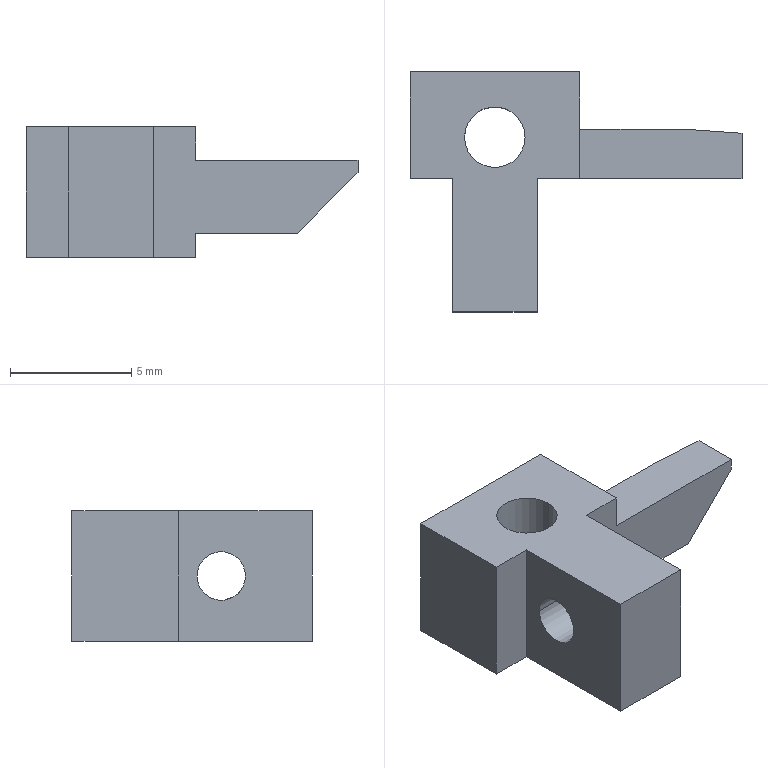Part | NX | 1 solid | 23 faces | box 13.7 x 9.913 x 5.4 mm | volume 252.029 mm3 | plane 17 | cylinder 6 | commonest cylinder face diameters 2 x2 2.5 x2 3.1 x2
STEP:
#1=CARTESIAN_POINT('',(-48.11,-45.316,4.403));
#2=VERTEX_POINT('',#1);
#3=CARTESIAN_POINT('',(-55.11,-45.316,4.403));
#4=VERTEX_POINT('',#3);
#5=CARTESIAN_POINT('',(-48.11,-45.316,4.403));
#6=DIRECTION('',(-1.,0.,0.));
#7=VECTOR('',#6,1000.);
#8=LINE('',#5,#7);
#9=EDGE_CURVE('',#2,#4,#8,.T.);
#10=ORIENTED_EDGE('',*,*,#9,.F.);
#11=CARTESIAN_POINT('',(-48.11,-45.316,-0.9969));
#12=VERTEX_POINT('',#11);
#13=CARTESIAN_POINT('',(-48.11,-45.316,4.403));
#14=DIRECTION('',(0.,0.,-1.));
#15=VECTOR('',#14,1000.);
#16=LINE('',#13,#15);
#17=EDGE_CURVE('',#2,#12,#16,.T.);
#18=ORIENTED_EDGE('',*,*,#17,.T.);
#19=CARTESIAN_POINT('',(-55.11,-45.316,-0.9969));
#20=VERTEX_POINT('',#19);
#21=CARTESIAN_POINT('',(-49.101,-45.316,-0.9969));
#22=DIRECTION('',(-1.,0.,0.));
#23=VECTOR('',#22,1000.);
#24=LINE('',#21,#23);
#25=EDGE_CURVE('',#12,#20,#24,.T.);
#26=ORIENTED_EDGE('',*,*,#25,.T.);
#27=CARTESIAN_POINT('',(-55.11,-45.316,4.403));
#28=DIRECTION('',(0.,0.,-1.));
#29=VECTOR('',#28,1000.);
#30=LINE('',#27,#29);
#31=EDGE_CURVE('',#4,#20,#30,.T.);
#32=ORIENTED_EDGE('',*,*,#31,.F.);
#33=EDGE_LOOP('',(#10,#18,#26,#32));
#34=FACE_BOUND('',#33,.T.);
#35=CARTESIAN_POINT('',(-48.11,-45.316,4.403));
#36=DIRECTION('',(0.,1.,0.));
#37=DIRECTION('',(0.,0.,-1.));
#38=AXIS2_PLACEMENT_3D('',#35,#36,#37);
#39=PLANE('',#38);
#40=ADVANCED_FACE('',(#34),#39,.T.);
#41=CARTESIAN_POINT('',(-48.11,-49.729,-0.9969));
#42=VERTEX_POINT('',#41);
#43=CARTESIAN_POINT('',(-48.11,-51.163,-0.9969));
#44=DIRECTION('',(0.,1.,0.));
#45=VECTOR('',#44,1000.);
#46=LINE('',#43,#45);
#47=EDGE_CURVE('',#42,#12,#46,.T.);
#48=ORIENTED_EDGE('',*,*,#47,.F.);
#49=CARTESIAN_POINT('',(-49.86,-49.729,-0.9969));
#50=VERTEX_POINT('',#49);
#51=CARTESIAN_POINT('',(-49.101,-49.729,-0.9969));
#52=DIRECTION('',(-1.,0.,0.));
#53=VECTOR('',#52,1000.);
#54=LINE('',#51,#53);
#55=EDGE_CURVE('',#42,#50,#54,.T.);
#56=ORIENTED_EDGE('',*,*,#55,.T.);
#57=CARTESIAN_POINT('',(-49.86,-55.229,-0.9969));
#58=VERTEX_POINT('',#57);
#59=CARTESIAN_POINT('',(-49.86,-51.163,-0.9969));
#60=DIRECTION('',(0.,-1.,0.));
#61=VECTOR('',#60,1000.);
#62=LINE('',#59,#61);
#63=EDGE_CURVE('',#50,#58,#62,.T.);
#64=ORIENTED_EDGE('',*,*,#63,.T.);
#65=CARTESIAN_POINT('',(-53.36,-55.229,-0.9969));
#66=VERTEX_POINT('',#65);
#67=CARTESIAN_POINT('',(-49.86,-55.229,-0.9969));
#68=DIRECTION('',(-1.,0.,0.));
#69=VECTOR('',#68,1000.);
#70=LINE('',#67,#69);
#71=EDGE_CURVE('',#58,#66,#70,.T.);
#72=ORIENTED_EDGE('',*,*,#71,.T.);
#73=CARTESIAN_POINT('',(-53.36,-49.729,-0.9969));
#74=VERTEX_POINT('',#73);
#75=CARTESIAN_POINT('',(-53.36,-51.163,-0.9969));
#76=DIRECTION('',(0.,-1.,0.));
#77=VECTOR('',#76,1000.);
#78=LINE('',#75,#77);
#79=EDGE_CURVE('',#74,#66,#78,.T.);
#80=ORIENTED_EDGE('',*,*,#79,.F.);
#81=CARTESIAN_POINT('',(-55.11,-49.729,-0.9969));
#82=VERTEX_POINT('',#81);
#83=CARTESIAN_POINT('',(-49.101,-49.729,-0.9969));
#84=DIRECTION('',(-1.,0.,0.));
#85=VECTOR('',#84,1000.);
#86=LINE('',#83,#85);
#87=EDGE_CURVE('',#74,#82,#86,.T.);
#88=ORIENTED_EDGE('',*,*,#87,.T.);
#89=CARTESIAN_POINT('',(-55.11,-51.163,-0.9969));
#90=DIRECTION('',(0.,1.,0.));
#91=VECTOR('',#90,1000.);
#92=LINE('',#89,#91);
#93=EDGE_CURVE('',#82,#20,#92,.T.);
#94=ORIENTED_EDGE('',*,*,#93,.T.);
#95=ORIENTED_EDGE('',*,*,#25,.F.);
#96=EDGE_LOOP('',(#48,#56,#64,#72,#80,#88,#94,#95));
#97=FACE_BOUND('',#96,.T.);
#98=CARTESIAN_POINT('',(-50.06,-53.51,-0.9969));
#99=VERTEX_POINT('',#98);
#100=CARTESIAN_POINT('',(-53.16,-53.51,-0.9969));
#101=VERTEX_POINT('',#100);
#102=CARTESIAN_POINT('',(-51.61,-53.51,-0.9969));
#103=DIRECTION('',(0.,0.,-1.));
#104=DIRECTION('',(-1.,0.,0.));
#105=AXIS2_PLACEMENT_3D('',#102,#103,#104);
#106=CIRCLE('',#105,1.55);
#107=EDGE_CURVE('',#99,#101,#106,.T.);
#108=ORIENTED_EDGE('',*,*,#107,.F.);
#109=CARTESIAN_POINT('',(-51.61,-53.51,-0.9969));
#110=DIRECTION('',(0.,0.,-1.));
#111=DIRECTION('',(-1.,0.,0.));
#112=AXIS2_PLACEMENT_3D('',#109,#110,#111);
#113=CIRCLE('',#112,1.55);
#114=EDGE_CURVE('',#101,#99,#113,.T.);
#115=ORIENTED_EDGE('',*,*,#114,.F.);
#116=EDGE_LOOP('',(#108,#115));
#117=FACE_BOUND('',#116,.T.);
#118=CARTESIAN_POINT('',(-52.86,-48.012,-0.9969));
#119=VERTEX_POINT('',#118);
#120=CARTESIAN_POINT('',(-50.36,-48.012,-0.9969));
#121=VERTEX_POINT('',#120);
#122=CARTESIAN_POINT('',(-51.61,-48.012,-0.9969));
#123=DIRECTION('',(0.,0.,-1.));
#124=DIRECTION('',(-1.,0.,0.));
#125=AXIS2_PLACEMENT_3D('',#122,#123,#124);
#126=CIRCLE('',#125,1.25);
#127=EDGE_CURVE('',#119,#121,#126,.T.);
#128=ORIENTED_EDGE('',*,*,#127,.F.);
#129=CARTESIAN_POINT('',(-51.61,-48.012,-0.9969));
#130=DIRECTION('',(0.,0.,-1.));
#131=DIRECTION('',(-1.,0.,0.));
#132=AXIS2_PLACEMENT_3D('',#129,#130,#131);
#133=CIRCLE('',#132,1.25);
#134=EDGE_CURVE('',#121,#119,#133,.T.);
#135=ORIENTED_EDGE('',*,*,#134,.F.);
#136=EDGE_LOOP('',(#128,#135));
#137=FACE_BOUND('',#136,.T.);
#138=CARTESIAN_POINT('',(-49.101,-51.163,-0.9969));
#139=DIRECTION('',(0.,0.,-1.));
#140=DIRECTION('',(0.,-1.,0.));
#141=AXIS2_PLACEMENT_3D('',#138,#139,#140);
#142=PLANE('',#141);
#143=ADVANCED_FACE('',(#97,#117,#137),#142,.T.);
#144=ORIENTED_EDGE('',*,*,#47,.T.);
#145=ORIENTED_EDGE('',*,*,#17,.F.);
#146=CARTESIAN_POINT('',(-48.11,-49.729,4.403));
#147=VERTEX_POINT('',#146);
#148=CARTESIAN_POINT('',(-48.11,-51.163,4.403));
#149=DIRECTION('',(0.,1.,0.));
#150=VECTOR('',#149,1000.);
#151=LINE('',#148,#150);
#152=EDGE_CURVE('',#147,#2,#151,.T.);
#153=ORIENTED_EDGE('',*,*,#152,.F.);
#154=CARTESIAN_POINT('',(-48.11,-49.729,3.003));
#155=VERTEX_POINT('',#154);
#156=CARTESIAN_POINT('',(-48.11,-49.729,4.403));
#157=DIRECTION('',(0.,0.,-1.));
#158=VECTOR('',#157,1000.);
#159=LINE('',#156,#158);
#160=EDGE_CURVE('',#147,#155,#159,.T.);
#161=ORIENTED_EDGE('',*,*,#160,.T.);
#162=CARTESIAN_POINT('',(-48.11,-47.687,3.003));
#163=VERTEX_POINT('',#162);
#164=CARTESIAN_POINT('',(-48.11,-51.163,3.003));
#165=DIRECTION('',(0.,-1.,0.));
#166=VECTOR('',#165,1000.);
#167=LINE('',#164,#166);
#168=EDGE_CURVE('',#163,#155,#167,.T.);
#169=ORIENTED_EDGE('',*,*,#168,.F.);
#170=CARTESIAN_POINT('',(-48.11,-47.687,0.003122));
#171=VERTEX_POINT('',#170);
#172=CARTESIAN_POINT('',(-48.11,-47.687,4.403));
#173=DIRECTION('',(0.,0.,1.));
#174=VECTOR('',#173,1000.);
#175=LINE('',#172,#174);
#176=EDGE_CURVE('',#171,#163,#175,.T.);
#177=ORIENTED_EDGE('',*,*,#176,.F.);
#178=CARTESIAN_POINT('',(-48.11,-49.729,0.003122));
#179=VERTEX_POINT('',#178);
#180=CARTESIAN_POINT('',(-48.11,-51.163,0.003122));
#181=DIRECTION('',(0.,1.,0.));
#182=VECTOR('',#181,1000.);
#183=LINE('',#180,#182);
#184=EDGE_CURVE('',#179,#171,#183,.T.);
#185=ORIENTED_EDGE('',*,*,#184,.F.);
#186=CARTESIAN_POINT('',(-48.11,-49.729,4.403));
#187=DIRECTION('',(0.,0.,-1.));
#188=VECTOR('',#187,1000.);
#189=LINE('',#186,#188);
#190=EDGE_CURVE('',#179,#42,#189,.T.);
#191=ORIENTED_EDGE('',*,*,#190,.T.);
#192=EDGE_LOOP('',(#144,#145,#153,#161,#169,#177,#185,#191));
#193=FACE_BOUND('',#192,.T.);
#194=CARTESIAN_POINT('',(-48.11,-47.529,-0.5969));
#195=DIRECTION('',(1.,0.,0.));
#196=DIRECTION('',(0.,1.,0.));
#197=AXIS2_PLACEMENT_3D('',#194,#195,#196);
#198=PLANE('',#197);
#199=ADVANCED_FACE('',(#193),#198,.T.);
#200=CARTESIAN_POINT('',(-55.11,-49.729,4.403));
#201=VERTEX_POINT('',#200);
#202=CARTESIAN_POINT('',(-55.11,-49.729,4.403));
#203=DIRECTION('',(0.,0.,1.));
#204=VECTOR('',#203,1000.);
#205=LINE('',#202,#204);
#206=EDGE_CURVE('',#82,#201,#205,.T.);
#207=ORIENTED_EDGE('',*,*,#206,.T.);
#208=CARTESIAN_POINT('',(-55.11,-51.163,4.403));
#209=DIRECTION('',(0.,-1.,0.));
#210=VECTOR('',#209,1000.);
#211=LINE('',#208,#210);
#212=EDGE_CURVE('',#4,#201,#211,.T.);
#213=ORIENTED_EDGE('',*,*,#212,.F.);
#214=ORIENTED_EDGE('',*,*,#31,.T.);
#215=ORIENTED_EDGE('',*,*,#93,.F.);
#216=EDGE_LOOP('',(#207,#213,#214,#215));
#217=FACE_BOUND('',#216,.T.);
#218=CARTESIAN_POINT('',(-55.11,-45.316,-0.5969));
#219=DIRECTION('',(-1.,0.,0.));
#220=DIRECTION('',(0.,0.,1.));
#221=AXIS2_PLACEMENT_3D('',#218,#219,#220);
#222=PLANE('',#221);
#223=ADVANCED_FACE('',(#217),#222,.T.);
#224=CARTESIAN_POINT('',(-43.739,-47.687,3.003));
#225=VERTEX_POINT('',#224);
#226=CARTESIAN_POINT('',(-49.101,-47.687,3.003));
#227=DIRECTION('',(1.,0.,0.));
#228=VECTOR('',#227,1000.);
#229=LINE('',#226,#228);
#230=EDGE_CURVE('',#163,#225,#229,.T.);
#231=ORIENTED_EDGE('',*,*,#230,.F.);
#232=ORIENTED_EDGE('',*,*,#168,.T.);
#233=CARTESIAN_POINT('',(-41.41,-49.729,3.003));
#234=VERTEX_POINT('',#233);
#235=CARTESIAN_POINT('',(-49.101,-49.729,3.003));
#236=DIRECTION('',(1.,0.,0.));
#237=VECTOR('',#236,1000.);
#238=LINE('',#235,#237);
#239=EDGE_CURVE('',#155,#234,#238,.T.);
#240=ORIENTED_EDGE('',*,*,#239,.T.);
#241=CARTESIAN_POINT('',(-41.41,-47.851,3.003));
#242=VERTEX_POINT('',#241);
#243=CARTESIAN_POINT('',(-41.41,-51.163,3.003));
#244=DIRECTION('',(0.,1.,0.));
#245=VECTOR('',#244,1000.);
#246=LINE('',#243,#245);
#247=EDGE_CURVE('',#234,#242,#246,.T.);
#248=ORIENTED_EDGE('',*,*,#247,.T.);
#249=CARTESIAN_POINT('',(-49.101,-47.307,3.003));
#250=DIRECTION('',(0.9975,-0.07053,0.));
#251=VECTOR('',#250,1000.);
#252=LINE('',#249,#251);
#253=EDGE_CURVE('',#225,#242,#252,.T.);
#254=ORIENTED_EDGE('',*,*,#253,.F.);
#255=EDGE_LOOP('',(#231,#232,#240,#248,#254));
#256=FACE_BOUND('',#255,.T.);
#257=CARTESIAN_POINT('',(-48.11,-53.629,3.003));
#258=DIRECTION('',(0.,0.,1.));
#259=DIRECTION('',(1.,0.,0.));
#260=AXIS2_PLACEMENT_3D('',#257,#258,#259);
#261=PLANE('',#260);
#262=ADVANCED_FACE('',(#256),#261,.T.);
#263=ORIENTED_EDGE('',*,*,#127,.T.);
#264=CARTESIAN_POINT('',(-50.36,-48.012,4.403));
#265=VERTEX_POINT('',#264);
#266=CARTESIAN_POINT('',(-50.36,-48.012,-2.597));
#267=DIRECTION('',(0.,0.,-1.));
#268=VECTOR('',#267,1000.);
#269=LINE('',#266,#268);
#270=EDGE_CURVE('',#265,#121,#269,.T.);
#271=ORIENTED_EDGE('',*,*,#270,.F.);
#272=CARTESIAN_POINT('',(-52.86,-48.012,4.403));
#273=VERTEX_POINT('',#272);
#274=CARTESIAN_POINT('',(-51.61,-48.012,4.403));
#275=DIRECTION('',(0.,0.,-1.));
#276=DIRECTION('',(-1.,0.,0.));
#277=AXIS2_PLACEMENT_3D('',#274,#275,#276);
#278=CIRCLE('',#277,1.25);
#279=EDGE_CURVE('',#273,#265,#278,.T.);
#280=ORIENTED_EDGE('',*,*,#279,.F.);
#281=CARTESIAN_POINT('',(-52.86,-48.012,-2.597));
#282=DIRECTION('',(0.,0.,-1.));
#283=VECTOR('',#282,1000.);
#284=LINE('',#281,#283);
#285=EDGE_CURVE('',#273,#119,#284,.T.);
#286=ORIENTED_EDGE('',*,*,#285,.T.);
#287=EDGE_LOOP('',(#263,#271,#280,#286));
#288=FACE_BOUND('',#287,.T.);
#289=CARTESIAN_POINT('',(-51.61,-48.012,-2.597));
#290=DIRECTION('',(0.,0.,-1.));
#291=DIRECTION('',(-1.,0.,0.));
#292=AXIS2_PLACEMENT_3D('',#289,#290,#291);
#293=CYLINDRICAL_SURFACE('',#292,1.25);
#294=ADVANCED_FACE('',(#288),#293,.F.);
#295=ORIENTED_EDGE('',*,*,#230,.T.);
#296=CARTESIAN_POINT('',(-46.739,-47.687,0.003122));
#297=VERTEX_POINT('',#296);
#298=CARTESIAN_POINT('',(-44.574,-47.687,2.167));
#299=DIRECTION('',(0.7071,0.,0.7071));
#300=VECTOR('',#299,1000.);
#301=LINE('',#298,#300);
#302=EDGE_CURVE('',#297,#225,#301,.T.);
#303=ORIENTED_EDGE('',*,*,#302,.F.);
#304=CARTESIAN_POINT('',(-49.101,-47.687,0.003122));
#305=DIRECTION('',(-1.,0.,0.));
#306=VECTOR('',#305,1000.);
#307=LINE('',#304,#306);
#308=EDGE_CURVE('',#297,#171,#307,.T.);
#309=ORIENTED_EDGE('',*,*,#308,.T.);
#310=ORIENTED_EDGE('',*,*,#176,.T.);
#311=EDGE_LOOP('',(#295,#303,#309,#310));
#312=FACE_BOUND('',#311,.T.);
#313=CARTESIAN_POINT('',(-48.11,-47.687,2.503));
#314=DIRECTION('',(0.,1.,0.));
#315=DIRECTION('',(1.,0.,0.));
#316=AXIS2_PLACEMENT_3D('',#313,#314,#315);
#317=PLANE('',#316);
#318=ADVANCED_FACE('',(#312),#317,.T.);
#319=ORIENTED_EDGE('',*,*,#87,.F.);
#320=CARTESIAN_POINT('',(-53.36,-49.729,4.403));
#321=VERTEX_POINT('',#320);
#322=CARTESIAN_POINT('',(-53.36,-49.729,4.403));
#323=DIRECTION('',(0.,0.,1.));
#324=VECTOR('',#323,1000.);
#325=LINE('',#322,#324);
#326=EDGE_CURVE('',#74,#321,#325,.T.);
#327=ORIENTED_EDGE('',*,*,#326,.T.);
#328=CARTESIAN_POINT('',(-49.101,-49.729,4.403));
#329=DIRECTION('',(-1.,0.,0.));
#330=VECTOR('',#329,1000.);
#331=LINE('',#328,#330);
#332=EDGE_CURVE('',#321,#201,#331,.T.);
#333=ORIENTED_EDGE('',*,*,#332,.T.);
#334=ORIENTED_EDGE('',*,*,#206,.F.);
#335=EDGE_LOOP('',(#319,#327,#333,#334));
#336=FACE_BOUND('',#335,.T.);
#337=CARTESIAN_POINT('',(-48.11,-49.729,-0.5969));
#338=DIRECTION('',(0.,-1.,0.));
#339=DIRECTION('',(0.,0.,-1.));
#340=AXIS2_PLACEMENT_3D('',#337,#338,#339);
#341=PLANE('',#340);
#342=ADVANCED_FACE('',(#336),#341,.T.);
#343=CARTESIAN_POINT('',(-41.41,-49.729,2.503));
#344=VERTEX_POINT('',#343);
#345=CARTESIAN_POINT('',(-41.41,-47.887,2.503));
#346=VERTEX_POINT('',#345);
#347=CARTESIAN_POINT('',(-41.41,-51.163,2.503));
#348=DIRECTION('',(0.,1.,0.));
#349=VECTOR('',#348,1000.);
#350=LINE('',#347,#349);
#351=EDGE_CURVE('',#344,#346,#350,.T.);
#352=ORIENTED_EDGE('',*,*,#351,.T.);
#353=CARTESIAN_POINT('',(-41.41,-47.752,4.403));
#354=DIRECTION('',(0.,-0.07053,-0.9975));
#355=VECTOR('',#354,1000.);
#356=LINE('',#353,#355);
#357=EDGE_CURVE('',#242,#346,#356,.T.);
#358=ORIENTED_EDGE('',*,*,#357,.F.);
#359=ORIENTED_EDGE('',*,*,#247,.F.);
#360=CARTESIAN_POINT('',(-41.41,-49.729,4.403));
#361=DIRECTION('',(0.,0.,-1.));
#362=VECTOR('',#361,1000.);
#363=LINE('',#360,#362);
#364=EDGE_CURVE('',#234,#344,#363,.T.);
#365=ORIENTED_EDGE('',*,*,#364,.T.);
#366=EDGE_LOOP('',(#352,#358,#359,#365));
#367=FACE_BOUND('',#366,.T.);
#368=CARTESIAN_POINT('',(-41.41,-49.37,2.047));
#369=DIRECTION('',(1.,0.,0.));
#370=DIRECTION('',(0.,1.,0.));
#371=AXIS2_PLACEMENT_3D('',#368,#369,#370);
#372=PLANE('',#371);
#373=ADVANCED_FACE('',(#367),#372,.T.);
#374=CARTESIAN_POINT('',(-43.91,-47.887,0.003122));
#375=VERTEX_POINT('',#374);
#376=CARTESIAN_POINT('',(-43.16,-47.887,0.7531));
#377=DIRECTION('',(0.7071,0.,0.7071));
#378=VECTOR('',#377,1000.);
#379=LINE('',#376,#378);
#380=EDGE_CURVE('',#375,#346,#379,.T.);
#381=ORIENTED_EDGE('',*,*,#380,.T.);
#382=ORIENTED_EDGE('',*,*,#351,.F.);
#383=CARTESIAN_POINT('',(-43.91,-49.729,0.003122));
#384=VERTEX_POINT('',#383);
#385=CARTESIAN_POINT('',(-39.51,-49.729,4.403));
#386=DIRECTION('',(-0.7071,0.,-0.7071));
#387=VECTOR('',#386,1000.);
#388=LINE('',#385,#387);
#389=EDGE_CURVE('',#344,#384,#388,.T.);
#390=ORIENTED_EDGE('',*,*,#389,.T.);
#391=CARTESIAN_POINT('',(-43.91,-51.163,0.003122));
#392=DIRECTION('',(0.,1.,0.));
#393=VECTOR('',#392,1000.);
#394=LINE('',#391,#393);
#395=EDGE_CURVE('',#384,#375,#394,.T.);
#396=ORIENTED_EDGE('',*,*,#395,.T.);
#397=EDGE_LOOP('',(#381,#382,#390,#396));
#398=FACE_BOUND('',#397,.T.);
#399=CARTESIAN_POINT('',(-43.16,-50.658,0.7531));
#400=DIRECTION('',(0.7071,0.,-0.7071));
#401=DIRECTION('',(0.,-1.,0.));
#402=AXIS2_PLACEMENT_3D('',#399,#400,#401);
#403=PLANE('',#402);
#404=ADVANCED_FACE('',(#398),#403,.T.);
#405=ORIENTED_EDGE('',*,*,#380,.F.);
#406=CARTESIAN_POINT('',(-49.101,-47.52,0.003122));
#407=DIRECTION('',(-0.9975,0.07053,0.));
#408=VECTOR('',#407,1000.);
#409=LINE('',#406,#408);
#410=EDGE_CURVE('',#375,#297,#409,.T.);
#411=ORIENTED_EDGE('',*,*,#410,.T.);
#412=ORIENTED_EDGE('',*,*,#302,.T.);
#413=ORIENTED_EDGE('',*,*,#253,.T.);
#414=ORIENTED_EDGE('',*,*,#357,.T.);
#415=EDGE_LOOP('',(#405,#411,#412,#413,#414));
#416=FACE_BOUND('',#415,.T.);
#417=CARTESIAN_POINT('',(-43.867,-47.787,1.46));
#418=DIRECTION('',(0.07036,0.995,-0.07036));
#419=DIRECTION('',(-0.7071,0.,-0.7071));
#420=AXIS2_PLACEMENT_3D('',#417,#418,#419);
#421=PLANE('',#420);
#422=ADVANCED_FACE('',(#416),#421,.T.);
#423=CARTESIAN_POINT('',(-49.101,-49.729,0.003122));
#424=DIRECTION('',(-1.,0.,0.));
#425=VECTOR('',#424,1000.);
#426=LINE('',#423,#425);
#427=EDGE_CURVE('',#384,#179,#426,.T.);
#428=ORIENTED_EDGE('',*,*,#427,.T.);
#429=ORIENTED_EDGE('',*,*,#184,.T.);
#430=ORIENTED_EDGE('',*,*,#308,.F.);
#431=ORIENTED_EDGE('',*,*,#410,.F.);
#432=ORIENTED_EDGE('',*,*,#395,.F.);
#433=EDGE_LOOP('',(#428,#429,#430,#431,#432));
#434=FACE_BOUND('',#433,.T.);
#435=CARTESIAN_POINT('',(-46.061,-49.047,0.003122));
#436=DIRECTION('',(0.,0.,-1.));
#437=DIRECTION('',(0.,-1.,0.));
#438=AXIS2_PLACEMENT_3D('',#435,#436,#437);
#439=PLANE('',#438);
#440=ADVANCED_FACE('',(#434),#439,.T.);
#441=CARTESIAN_POINT('',(-49.86,-49.729,4.403));
#442=VERTEX_POINT('',#441);
#443=CARTESIAN_POINT('',(-49.86,-49.729,4.403));
#444=DIRECTION('',(0.,0.,-1.));
#445=VECTOR('',#444,1000.);
#446=LINE('',#443,#445);
#447=EDGE_CURVE('',#442,#50,#446,.T.);
#448=ORIENTED_EDGE('',*,*,#447,.T.);
#449=ORIENTED_EDGE('',*,*,#55,.F.);
#450=ORIENTED_EDGE('',*,*,#190,.F.);
#451=ORIENTED_EDGE('',*,*,#427,.F.);
#452=ORIENTED_EDGE('',*,*,#389,.F.);
#453=ORIENTED_EDGE('',*,*,#364,.F.);
#454=ORIENTED_EDGE('',*,*,#239,.F.);
#455=ORIENTED_EDGE('',*,*,#160,.F.);
#456=CARTESIAN_POINT('',(-49.101,-49.729,4.403));
#457=DIRECTION('',(-1.,0.,0.));
#458=VECTOR('',#457,1000.);
#459=LINE('',#456,#458);
#460=EDGE_CURVE('',#147,#442,#459,.T.);
#461=ORIENTED_EDGE('',*,*,#460,.T.);
#462=EDGE_LOOP('',(#448,#449,#450,#451,#452,#453,#454,#455,#461));
#463=FACE_BOUND('',#462,.T.);
#464=CARTESIAN_POINT('',(-48.11,-49.729,-0.5969));
#465=DIRECTION('',(0.,-1.,0.));
#466=DIRECTION('',(0.,0.,-1.));
#467=AXIS2_PLACEMENT_3D('',#464,#465,#466);
#468=PLANE('',#467);
#469=ADVANCED_FACE('',(#463),#468,.T.);
#470=ORIENTED_EDGE('',*,*,#326,.F.);
#471=ORIENTED_EDGE('',*,*,#79,.T.);
#472=CARTESIAN_POINT('',(-53.36,-55.229,4.403));
#473=VERTEX_POINT('',#472);
#474=CARTESIAN_POINT('',(-53.36,-55.229,-0.9969));
#475=DIRECTION('',(0.,0.,1.));
#476=VECTOR('',#475,1000.);
#477=LINE('',#474,#476);
#478=EDGE_CURVE('',#66,#473,#477,.T.);
#479=ORIENTED_EDGE('',*,*,#478,.T.);
#480=CARTESIAN_POINT('',(-53.36,-51.163,4.403));
#481=DIRECTION('',(0.,-1.,0.));
#482=VECTOR('',#481,1000.);
#483=LINE('',#480,#482);
#484=EDGE_CURVE('',#321,#473,#483,.T.);
#485=ORIENTED_EDGE('',*,*,#484,.F.);
#486=EDGE_LOOP('',(#470,#471,#479,#485));
#487=FACE_BOUND('',#486,.T.);
#488=CARTESIAN_POINT('',(-53.36,-50.479,1.703));
#489=VERTEX_POINT('',#488);
#490=CARTESIAN_POINT('',(-53.36,-52.479,1.703));
#491=VERTEX_POINT('',#490);
#492=CARTESIAN_POINT('',(-53.36,-51.479,1.703));
#493=DIRECTION('',(-1.,0.,0.));
#494=DIRECTION('',(0.,-1.,0.));
#495=AXIS2_PLACEMENT_3D('',#492,#493,#494);
#496=CIRCLE('',#495,1.);
#497=EDGE_CURVE('',#489,#491,#496,.T.);
#498=ORIENTED_EDGE('',*,*,#497,.F.);
#499=CARTESIAN_POINT('',(-53.36,-51.479,1.703));
#500=DIRECTION('',(-1.,0.,0.));
#501=DIRECTION('',(0.,-1.,0.));
#502=AXIS2_PLACEMENT_3D('',#499,#500,#501);
#503=CIRCLE('',#502,1.);
#504=EDGE_CURVE('',#491,#489,#503,.T.);
#505=ORIENTED_EDGE('',*,*,#504,.F.);
#506=EDGE_LOOP('',(#498,#505));
#507=FACE_BOUND('',#506,.T.);
#508=CARTESIAN_POINT('',(-53.36,-50.229,-0.9969));
#509=DIRECTION('',(-1.,0.,0.));
#510=DIRECTION('',(0.,0.,1.));
#511=AXIS2_PLACEMENT_3D('',#508,#509,#510);
#512=PLANE('',#511);
#513=ADVANCED_FACE('',(#487,#507),#512,.T.);
#514=ORIENTED_EDGE('',*,*,#447,.F.);
#515=CARTESIAN_POINT('',(-49.86,-55.229,4.403));
#516=VERTEX_POINT('',#515);
#517=CARTESIAN_POINT('',(-49.86,-51.163,4.403));
#518=DIRECTION('',(0.,-1.,0.));
#519=VECTOR('',#518,1000.);
#520=LINE('',#517,#519);
#521=EDGE_CURVE('',#442,#516,#520,.T.);
#522=ORIENTED_EDGE('',*,*,#521,.T.);
#523=CARTESIAN_POINT('',(-49.86,-55.229,4.403));
#524=DIRECTION('',(0.,0.,-1.));
#525=VECTOR('',#524,1000.);
#526=LINE('',#523,#525);
#527=EDGE_CURVE('',#516,#58,#526,.T.);
#528=ORIENTED_EDGE('',*,*,#527,.T.);
#529=ORIENTED_EDGE('',*,*,#63,.F.);
#530=EDGE_LOOP('',(#514,#522,#528,#529));
#531=FACE_BOUND('',#530,.T.);
#532=CARTESIAN_POINT('',(-49.86,-52.479,1.703));
#533=VERTEX_POINT('',#532);
#534=CARTESIAN_POINT('',(-49.86,-50.479,1.703));
#535=VERTEX_POINT('',#534);
#536=CARTESIAN_POINT('',(-49.86,-51.479,1.703));
#537=DIRECTION('',(-1.,0.,0.));
#538=DIRECTION('',(0.,-1.,0.));
#539=AXIS2_PLACEMENT_3D('',#536,#537,#538);
#540=CIRCLE('',#539,1.);
#541=EDGE_CURVE('',#533,#535,#540,.T.);
#542=ORIENTED_EDGE('',*,*,#541,.T.);
#543=CARTESIAN_POINT('',(-49.86,-51.479,1.703));
#544=DIRECTION('',(-1.,0.,0.));
#545=DIRECTION('',(0.,-1.,0.));
#546=AXIS2_PLACEMENT_3D('',#543,#544,#545);
#547=CIRCLE('',#546,1.);
#548=EDGE_CURVE('',#535,#533,#547,.T.);
#549=ORIENTED_EDGE('',*,*,#548,.T.);
#550=EDGE_LOOP('',(#542,#549));
#551=FACE_BOUND('',#550,.T.);
#552=CARTESIAN_POINT('',(-49.86,-50.229,4.403));
#553=DIRECTION('',(1.,0.,0.));
#554=DIRECTION('',(0.,1.,0.));
#555=AXIS2_PLACEMENT_3D('',#552,#553,#554);
#556=PLANE('',#555);
#557=ADVANCED_FACE('',(#531,#551),#556,.T.);
#558=ORIENTED_EDGE('',*,*,#478,.F.);
#559=ORIENTED_EDGE('',*,*,#71,.F.);
#560=ORIENTED_EDGE('',*,*,#527,.F.);
#561=CARTESIAN_POINT('',(-53.36,-55.229,4.403));
#562=DIRECTION('',(1.,0.,0.));
#563=VECTOR('',#562,1000.);
#564=LINE('',#561,#563);
#565=EDGE_CURVE('',#473,#516,#564,.T.);
#566=ORIENTED_EDGE('',*,*,#565,.F.);
#567=EDGE_LOOP('',(#558,#559,#560,#566));
#568=FACE_BOUND('',#567,.T.);
#569=CARTESIAN_POINT('',(-51.674,-55.229,-0.05073));
#570=DIRECTION('',(0.,-1.,0.));
#571=DIRECTION('',(0.,0.,-1.));
#572=AXIS2_PLACEMENT_3D('',#569,#570,#571);
#573=PLANE('',#572);
#574=ADVANCED_FACE('',(#568),#573,.T.);
#575=ORIENTED_EDGE('',*,*,#497,.T.);
#576=CARTESIAN_POINT('',(-40.04,-52.479,1.703));
#577=DIRECTION('',(-1.,0.,0.));
#578=VECTOR('',#577,1000.);
#579=LINE('',#576,#578);
#580=EDGE_CURVE('',#491,#533,#579,.F.);
#581=ORIENTED_EDGE('',*,*,#580,.T.);
#582=ORIENTED_EDGE('',*,*,#548,.F.);
#583=CARTESIAN_POINT('',(-40.04,-50.479,1.703));
#584=DIRECTION('',(-1.,0.,0.));
#585=VECTOR('',#584,1000.);
#586=LINE('',#583,#585);
#587=EDGE_CURVE('',#489,#535,#586,.F.);
#588=ORIENTED_EDGE('',*,*,#587,.F.);
#589=EDGE_LOOP('',(#575,#581,#582,#588));
#590=FACE_BOUND('',#589,.T.);
#591=CARTESIAN_POINT('',(-52.427,-52.193,1.003));
#592=VERTEX_POINT('',#591);
#593=CARTESIAN_POINT('',(-50.793,-52.193,1.003));
#594=VERTEX_POINT('',#593);
#595=CARTESIAN_POINT('',(-52.427,-52.193,1.003));
#596=CARTESIAN_POINT('',(-52.414,-52.185,0.9943));
#597=CARTESIAN_POINT('',(-52.399,-52.176,0.986));
#598=CARTESIAN_POINT('',(-52.385,-52.168,0.9781));
#599=CARTESIAN_POINT('',(-52.37,-52.159,0.9701));
#600=CARTESIAN_POINT('',(-52.356,-52.151,0.9626));
#601=CARTESIAN_POINT('',(-52.341,-52.143,0.9555));
#602=CARTESIAN_POINT('',(-52.326,-52.135,0.9484));
#603=CARTESIAN_POINT('',(-52.311,-52.127,0.9417));
#604=CARTESIAN_POINT('',(-52.295,-52.12,0.9353));
#605=CARTESIAN_POINT('',(-52.28,-52.112,0.929));
#606=CARTESIAN_POINT('',(-52.264,-52.105,0.923));
#607=CARTESIAN_POINT('',(-52.248,-52.097,0.9173));
#608=CARTESIAN_POINT('',(-52.232,-52.09,0.9116));
#609=CARTESIAN_POINT('',(-52.215,-52.083,0.9062));
#610=CARTESIAN_POINT('',(-52.199,-52.076,0.9012));
#611=CARTESIAN_POINT('',(-52.183,-52.07,0.8962));
#612=CARTESIAN_POINT('',(-52.166,-52.063,0.8914));
#613=CARTESIAN_POINT('',(-52.149,-52.057,0.887));
#614=CARTESIAN_POINT('',(-52.132,-52.051,0.8826));
#615=CARTESIAN_POINT('',(-52.115,-52.045,0.8785));
#616=CARTESIAN_POINT('',(-52.098,-52.039,0.8746));
#617=CARTESIAN_POINT('',(-52.081,-52.033,0.8708));
#618=CARTESIAN_POINT('',(-52.063,-52.028,0.8672));
#619=CARTESIAN_POINT('',(-52.046,-52.023,0.8639));
#620=CARTESIAN_POINT('',(-52.029,-52.018,0.8606));
#621=CARTESIAN_POINT('',(-52.011,-52.013,0.8575));
#622=CARTESIAN_POINT('',(-51.993,-52.008,0.8547));
#623=CARTESIAN_POINT('',(-51.976,-52.004,0.8519));
#624=CARTESIAN_POINT('',(-51.958,-52.,0.8494));
#625=CARTESIAN_POINT('',(-51.94,-51.996,0.847));
#626=CARTESIAN_POINT('',(-51.905,-51.988,0.8423));
#627=CARTESIAN_POINT('',(-51.868,-51.981,0.8385));
#628=CARTESIAN_POINT('',(-51.832,-51.976,0.8355));
#629=CARTESIAN_POINT('',(-51.795,-51.971,0.8324));
#630=CARTESIAN_POINT('',(-51.758,-51.967,0.8302));
#631=CARTESIAN_POINT('',(-51.721,-51.964,0.8287));
#632=CARTESIAN_POINT('',(-51.685,-51.962,0.8273));
#633=CARTESIAN_POINT('',(-51.647,-51.96,0.8265));
#634=CARTESIAN_POINT('',(-51.61,-51.96,0.8265));
#635=CARTESIAN_POINT('',(-51.573,-51.96,0.8265));
#636=CARTESIAN_POINT('',(-51.536,-51.962,0.8273));
#637=CARTESIAN_POINT('',(-51.5,-51.964,0.8287));
#638=CARTESIAN_POINT('',(-51.481,-51.965,0.8294));
#639=CARTESIAN_POINT('',(-51.463,-51.967,0.8304));
#640=CARTESIAN_POINT('',(-51.445,-51.969,0.8315));
#641=CARTESIAN_POINT('',(-51.427,-51.971,0.8326));
#642=CARTESIAN_POINT('',(-51.408,-51.973,0.8339));
#643=CARTESIAN_POINT('',(-51.39,-51.976,0.8354));
#644=CARTESIAN_POINT('',(-51.372,-51.979,0.8369));
#645=CARTESIAN_POINT('',(-51.354,-51.981,0.8386));
#646=CARTESIAN_POINT('',(-51.335,-51.985,0.8405));
#647=CARTESIAN_POINT('',(-51.317,-51.988,0.8424));
#648=CARTESIAN_POINT('',(-51.299,-51.992,0.8445));
#649=CARTESIAN_POINT('',(-51.281,-51.996,0.8469));
#650=CARTESIAN_POINT('',(-51.263,-51.999,0.8492));
#651=CARTESIAN_POINT('',(-51.245,-52.004,0.8518));
#652=CARTESIAN_POINT('',(-51.228,-52.008,0.8546));
#653=CARTESIAN_POINT('',(-51.21,-52.013,0.8574));
#654=CARTESIAN_POINT('',(-51.192,-52.018,0.8605));
#655=CARTESIAN_POINT('',(-51.175,-52.023,0.8638));
#656=CARTESIAN_POINT('',(-51.157,-52.028,0.8671));
#657=CARTESIAN_POINT('',(-51.14,-52.033,0.8707));
#658=CARTESIAN_POINT('',(-51.123,-52.039,0.8746));
#659=CARTESIAN_POINT('',(-51.106,-52.045,0.8784));
#660=CARTESIAN_POINT('',(-51.089,-52.051,0.8825));
#661=CARTESIAN_POINT('',(-51.072,-52.057,0.8869));
#662=CARTESIAN_POINT('',(-51.055,-52.063,0.8913));
#663=CARTESIAN_POINT('',(-51.038,-52.069,0.896));
#664=CARTESIAN_POINT('',(-51.022,-52.076,0.901));
#665=CARTESIAN_POINT('',(-51.006,-52.083,0.906));
#666=CARTESIAN_POINT('',(-50.99,-52.09,0.9113));
#667=CARTESIAN_POINT('',(-50.974,-52.097,0.917));
#668=CARTESIAN_POINT('',(-50.958,-52.104,0.9227));
#669=CARTESIAN_POINT('',(-50.942,-52.112,0.9287));
#670=CARTESIAN_POINT('',(-50.926,-52.119,0.9351));
#671=CARTESIAN_POINT('',(-50.91,-52.127,0.9415));
#672=CARTESIAN_POINT('',(-50.895,-52.135,0.9483));
#673=CARTESIAN_POINT('',(-50.88,-52.143,0.9554));
#674=CARTESIAN_POINT('',(-50.865,-52.151,0.9626));
#675=CARTESIAN_POINT('',(-50.85,-52.159,0.9701));
#676=CARTESIAN_POINT('',(-50.836,-52.168,0.9781));
#677=CARTESIAN_POINT('',(-50.821,-52.176,0.986));
#678=CARTESIAN_POINT('',(-50.807,-52.185,0.9944));
#679=CARTESIAN_POINT('',(-50.793,-52.193,1.003));
#680=B_SPLINE_CURVE_WITH_KNOTS('',3,(#595,#596,#597,#598,#599,#600,#601,#602,#603,#604,#605,#606,#607,#608,#609,#610,#611,#612,#613,#614,#615,#616,#617,#618,#619,#620,#621,#622,#623,#624,#625,#626,#627,#628,#629,#630,#631,#632,#633,#634,#635,#636,#637,#638,#639,#640,#641,#642,#643,#644,#645,#646,#647,#648,#649,#650,#651,#652,#653,#654,#655,#656,#657,#658,#659,#660,#661,#662,#663,#664,#665,#666,#667,#668,#669,#670,#671,#672,#673,#674,#675,#676,#677,#678,#679),.UNSPECIFIED.,.F.,.F.,(4,3,3,3,3,3,3,3,3,3,3,3,3,3,3,3,3,3,3,3,3,3,3,3,3,3,3,3,4),(0.,0.05553,0.1109,0.1661,0.2214,0.2768,0.3323,0.3878,0.4433,0.4986,0.5538,0.6646,0.7758,0.887,0.9978,1.053,1.108,1.164,1.22,1.275,1.331,1.386,1.442,1.497,1.552,1.608,1.663,1.719,1.774),.UNSPECIFIED.);
#681=EDGE_CURVE('',#592,#594,#680,.T.);
#682=ORIENTED_EDGE('',*,*,#681,.T.);
#683=CARTESIAN_POINT('',(-40.04,-52.193,1.003));
#684=DIRECTION('',(-1.,0.,0.));
#685=VECTOR('',#684,1000.);
#686=LINE('',#683,#685);
#687=EDGE_CURVE('',#594,#592,#686,.T.);
#688=ORIENTED_EDGE('',*,*,#687,.T.);
#689=EDGE_LOOP('',(#682,#688));
#690=FACE_BOUND('',#689,.T.);
#691=CARTESIAN_POINT('',(-40.04,-51.479,1.703));
#692=DIRECTION('',(-1.,0.,0.));
#693=DIRECTION('',(0.,-1.,0.));
#694=AXIS2_PLACEMENT_3D('',#691,#692,#693);
#695=CYLINDRICAL_SURFACE('',#694,1.);
#696=ADVANCED_FACE('',(#590,#690),#695,.F.);
#697=CARTESIAN_POINT('',(-53.16,-53.51,1.003));
#698=VERTEX_POINT('',#697);
#699=CARTESIAN_POINT('',(-51.61,-53.51,1.003));
#700=DIRECTION('',(0.,0.,-1.));
#701=DIRECTION('',(-1.,0.,0.));
#702=AXIS2_PLACEMENT_3D('',#699,#700,#701);
#703=CIRCLE('',#702,1.55);
#704=EDGE_CURVE('',#698,#592,#703,.T.);
#705=ORIENTED_EDGE('',*,*,#704,.T.);
#706=ORIENTED_EDGE('',*,*,#687,.F.);
#707=CARTESIAN_POINT('',(-50.06,-53.51,1.003));
#708=VERTEX_POINT('',#707);
#709=CARTESIAN_POINT('',(-51.61,-53.51,1.003));
#710=DIRECTION('',(0.,0.,-1.));
#711=DIRECTION('',(-1.,0.,0.));
#712=AXIS2_PLACEMENT_3D('',#709,#710,#711);
#713=CIRCLE('',#712,1.55);
#714=EDGE_CURVE('',#594,#708,#713,.T.);
#715=ORIENTED_EDGE('',*,*,#714,.T.);
#716=CARTESIAN_POINT('',(-51.61,-53.51,1.003));
#717=DIRECTION('',(0.,0.,-1.));
#718=DIRECTION('',(-1.,0.,0.));
#719=AXIS2_PLACEMENT_3D('',#716,#717,#718);
#720=CIRCLE('',#719,1.55);
#721=EDGE_CURVE('',#708,#698,#720,.T.);
#722=ORIENTED_EDGE('',*,*,#721,.T.);
#723=EDGE_LOOP('',(#705,#706,#715,#722));
#724=FACE_BOUND('',#723,.T.);
#725=CARTESIAN_POINT('',(-51.111,-53.01,1.003));
#726=DIRECTION('',(0.,0.,-1.));
#727=DIRECTION('',(0.,-1.,0.));
#728=AXIS2_PLACEMENT_3D('',#725,#726,#727);
#729=PLANE('',#728);
#730=ADVANCED_FACE('',(#724),#729,.T.);
#731=ORIENTED_EDGE('',*,*,#704,.F.);
#732=CARTESIAN_POINT('',(-53.16,-53.51,-0.9969));
#733=DIRECTION('',(0.,0.,-1.));
#734=VECTOR('',#733,1000.);
#735=LINE('',#732,#734);
#736=EDGE_CURVE('',#101,#698,#735,.F.);
#737=ORIENTED_EDGE('',*,*,#736,.F.);
#738=ORIENTED_EDGE('',*,*,#114,.T.);
#739=CARTESIAN_POINT('',(-50.06,-53.51,-0.9969));
#740=DIRECTION('',(0.,0.,-1.));
#741=VECTOR('',#740,1000.);
#742=LINE('',#739,#741);
#743=EDGE_CURVE('',#99,#708,#742,.F.);
#744=ORIENTED_EDGE('',*,*,#743,.T.);
#745=ORIENTED_EDGE('',*,*,#714,.F.);
#746=ORIENTED_EDGE('',*,*,#681,.F.);
#747=EDGE_LOOP('',(#731,#737,#738,#744,#745,#746));
#748=FACE_BOUND('',#747,.T.);
#749=CARTESIAN_POINT('',(-51.61,-53.51,-0.9969));
#750=DIRECTION('',(0.,0.,-1.));
#751=DIRECTION('',(-1.,0.,0.));
#752=AXIS2_PLACEMENT_3D('',#749,#750,#751);
#753=CYLINDRICAL_SURFACE('',#752,1.55);
#754=ADVANCED_FACE('',(#748),#753,.F.);
#755=ORIENTED_EDGE('',*,*,#332,.F.);
#756=ORIENTED_EDGE('',*,*,#484,.T.);
#757=ORIENTED_EDGE('',*,*,#565,.T.);
#758=ORIENTED_EDGE('',*,*,#521,.F.);
#759=ORIENTED_EDGE('',*,*,#460,.F.);
#760=ORIENTED_EDGE('',*,*,#152,.T.);
#761=ORIENTED_EDGE('',*,*,#9,.T.);
#762=ORIENTED_EDGE('',*,*,#212,.T.);
#763=EDGE_LOOP('',(#755,#756,#757,#758,#759,#760,#761,#762));
#764=FACE_BOUND('',#763,.T.);
#765=CARTESIAN_POINT('',(-51.61,-48.012,4.403));
#766=DIRECTION('',(0.,0.,-1.));
#767=DIRECTION('',(-1.,0.,0.));
#768=AXIS2_PLACEMENT_3D('',#765,#766,#767);
#769=CIRCLE('',#768,1.25);
#770=EDGE_CURVE('',#265,#273,#769,.T.);
#771=ORIENTED_EDGE('',*,*,#770,.T.);
#772=ORIENTED_EDGE('',*,*,#279,.T.);
#773=EDGE_LOOP('',(#771,#772));
#774=FACE_BOUND('',#773,.T.);
#775=CARTESIAN_POINT('',(-49.101,-51.163,4.403));
#776=DIRECTION('',(0.,0.,-1.));
#777=DIRECTION('',(0.,-1.,0.));
#778=AXIS2_PLACEMENT_3D('',#775,#776,#777);
#779=PLANE('',#778);
#780=ADVANCED_FACE('',(#764,#774),#779,.F.);
#781=ORIENTED_EDGE('',*,*,#541,.F.);
#782=ORIENTED_EDGE('',*,*,#580,.F.);
#783=ORIENTED_EDGE('',*,*,#504,.T.);
#784=ORIENTED_EDGE('',*,*,#587,.T.);
#785=EDGE_LOOP('',(#781,#782,#783,#784));
#786=FACE_BOUND('',#785,.T.);
#787=CARTESIAN_POINT('',(-40.04,-51.479,1.703));
#788=DIRECTION('',(-1.,0.,0.));
#789=DIRECTION('',(0.,-1.,0.));
#790=AXIS2_PLACEMENT_3D('',#787,#788,#789);
#791=CYLINDRICAL_SURFACE('',#790,1.);
#792=ADVANCED_FACE('',(#786),#791,.F.);
#793=ORIENTED_EDGE('',*,*,#107,.T.);
#794=ORIENTED_EDGE('',*,*,#736,.T.);
#795=ORIENTED_EDGE('',*,*,#721,.F.);
#796=ORIENTED_EDGE('',*,*,#743,.F.);
#797=EDGE_LOOP('',(#793,#794,#795,#796));
#798=FACE_BOUND('',#797,.T.);
#799=CARTESIAN_POINT('',(-51.61,-53.51,-0.9969));
#800=DIRECTION('',(0.,0.,-1.));
#801=DIRECTION('',(-1.,0.,0.));
#802=AXIS2_PLACEMENT_3D('',#799,#800,#801);
#803=CYLINDRICAL_SURFACE('',#802,1.55);
#804=ADVANCED_FACE('',(#798),#803,.F.);
#805=ORIENTED_EDGE('',*,*,#770,.F.);
#806=ORIENTED_EDGE('',*,*,#270,.T.);
#807=ORIENTED_EDGE('',*,*,#134,.T.);
#808=ORIENTED_EDGE('',*,*,#285,.F.);
#809=EDGE_LOOP('',(#805,#806,#807,#808));
#810=FACE_BOUND('',#809,.T.);
#811=CARTESIAN_POINT('',(-51.61,-48.012,-2.597));
#812=DIRECTION('',(0.,0.,-1.));
#813=DIRECTION('',(-1.,0.,0.));
#814=AXIS2_PLACEMENT_3D('',#811,#812,#813);
#815=CYLINDRICAL_SURFACE('',#814,1.25);
#816=ADVANCED_FACE('',(#810),#815,.F.);
#817=CLOSED_SHELL('',(#40,#143,#199,#223,#262,#294,#318,#342,#373,#404,#422,#440,#469,#513,#557,#574,#696,#730,#754,#780,#792,#804,#816));
#818=MANIFOLD_SOLID_BREP('',#817);
#819=(LENGTH_UNIT()NAMED_UNIT(*)SI_UNIT(.MILLI.,.METRE.));
#820=UNCERTAINTY_MEASURE_WITH_UNIT(LENGTH_MEASURE(0.00001),#819,'','');
#821=(NAMED_UNIT(*)PLANE_ANGLE_UNIT()SI_UNIT($,.RADIAN.));
#822=(NAMED_UNIT(*)SI_UNIT($,.STERADIAN.)SOLID_ANGLE_UNIT());
#823=(GEOMETRIC_REPRESENTATION_CONTEXT(3)GLOBAL_UNCERTAINTY_ASSIGNED_CONTEXT((#820))GLOBAL_UNIT_ASSIGNED_CONTEXT((#819,#821,#822))REPRESENTATION_CONTEXT('',''));
#824=ADVANCED_BREP_SHAPE_REPRESENTATION('',(#818),#823);